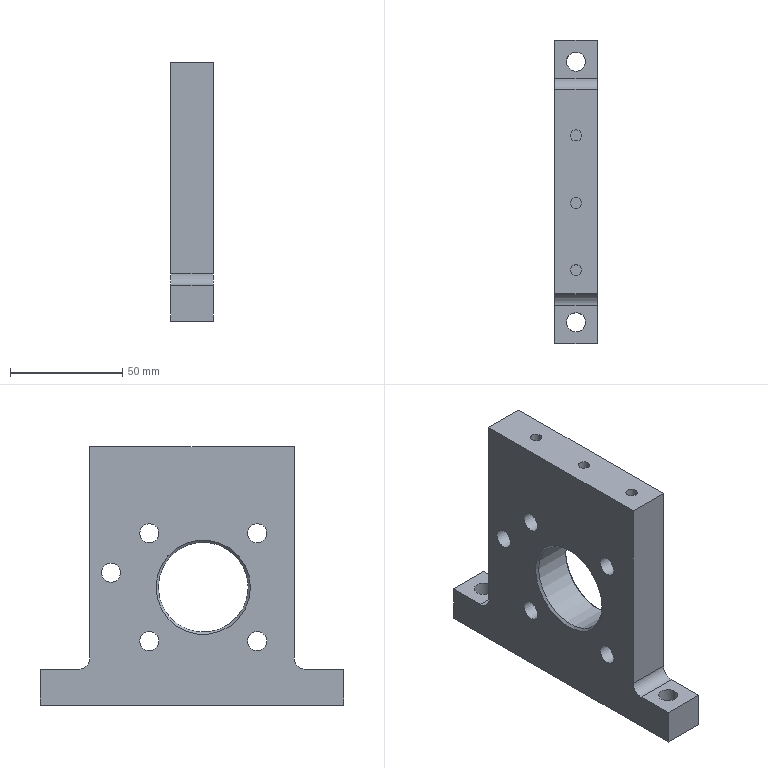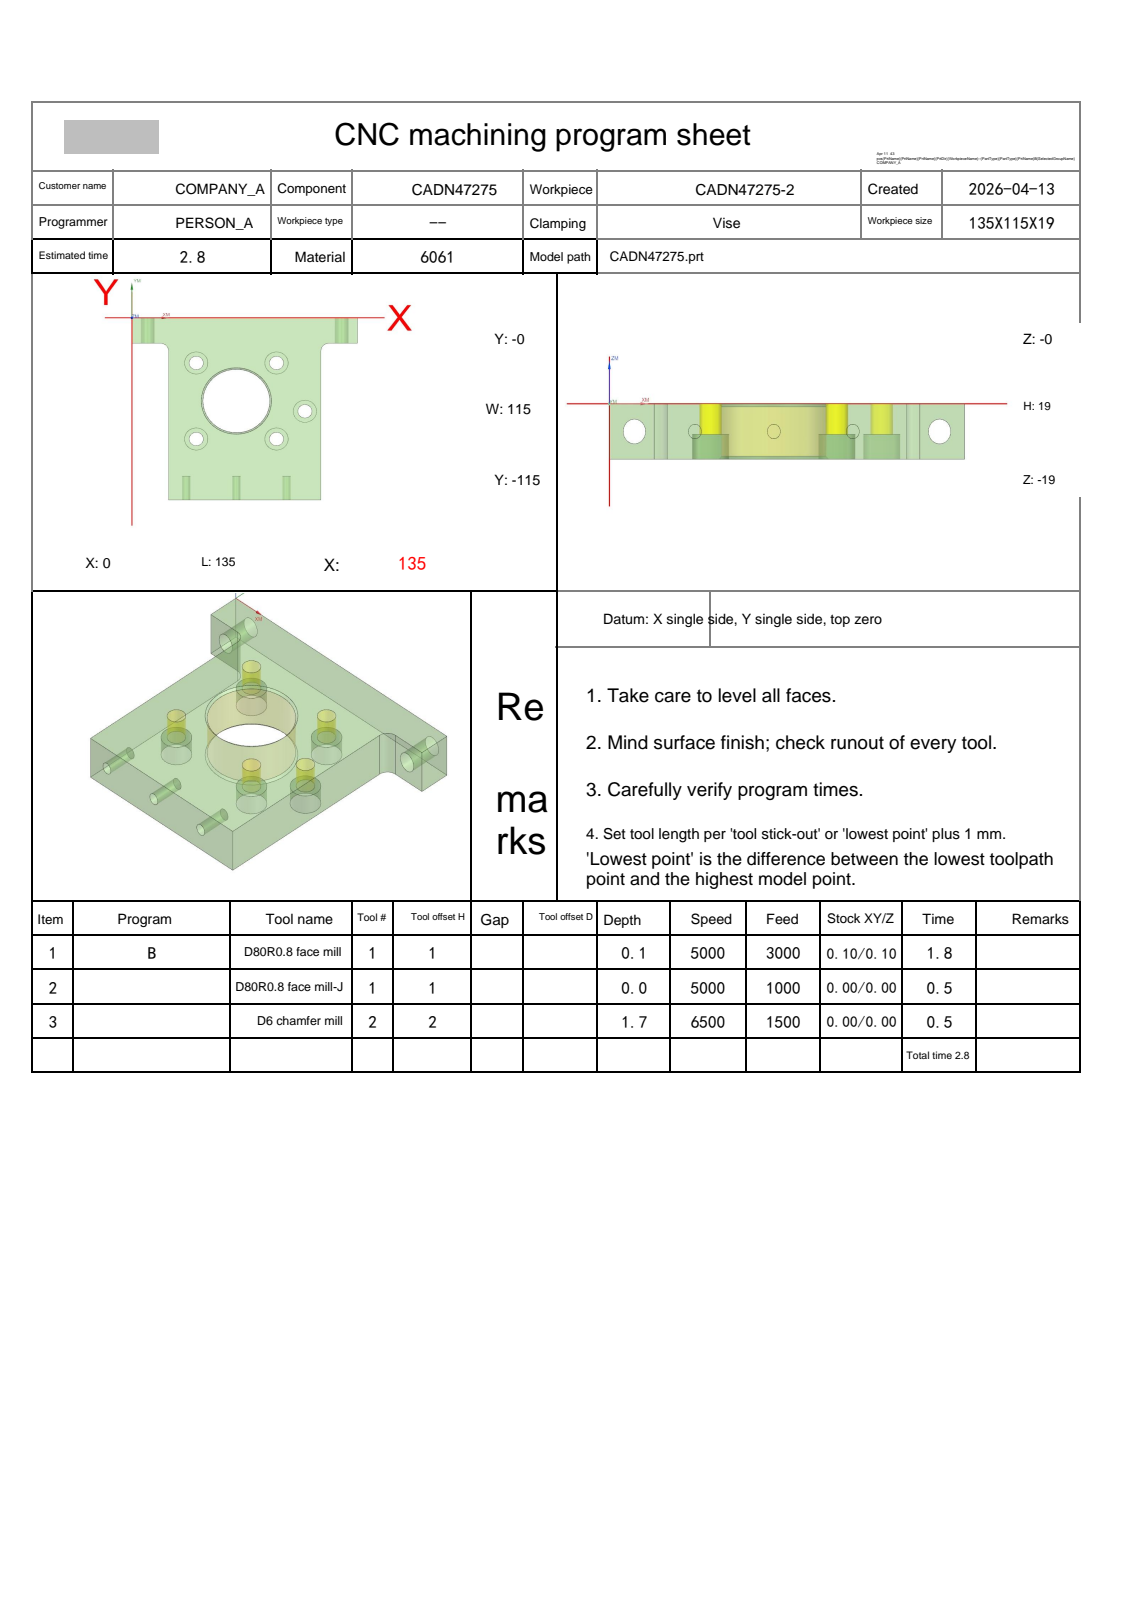NC program | NX | posted by the shop | part box 19 x 135 x 115 mm
Whole program:
%
O0001
(Machine time: 3.42 MIN)
(===Total Tool:2===)
(T1=D80R0.8 face mill D=80.  R=0.8  D-  H01 Z=-0.   )
(T2=D6 chamfer mill   D=6.   R=0.   D-  H02 Z=-1.7  )
G80 G90 G17 G49 G40
G91 G28 Z0
M01
N1 T01 M06
(D80R0.8 face mill  D=80. R=0.8 H=01 ce=0.10 di=0.10)
G00 G90 G54 X-52.097 Y-23.903 M03 S5000
G43 H01 Z20.
M08
Z7.009
G01 Z5.009 F3000.
X-40.097
X167.1
G02 X175.097 Y-31.9 I-.003 J-8.
G01 Y-53.303
G02 X173.357 Y-58.283 I-8. J.001
G01 X155.497 Y-80.721
G02 X149.243 Y-83.737 I-6.258 J4.984
G01 X-18.097
X-30.097
Z7.009
G00 X-52.097 Y-23.903
Z6.518
G01 Z4.518
X-40.097
X167.1
G02 X175.097 Y-31.9 I-.003 J-8.
G01 Y-53.303
G02 X173.357 Y-58.283 I-8. J.001
G01 X155.497 Y-80.721
G02 X149.243 Y-83.737 I-6.258 J4.984
G01 X-18.097
X-30.097
Z6.518
G00 X-52.097 Y-23.903
Z6.027
G01 Z4.027
X-40.097
X167.1
G02 X175.097 Y-31.9 I-.003 J-8.
G01 Y-53.303
G02 X173.357 Y-58.283 I-8. J.001
G01 X155.497 Y-80.721
G02 X149.243 Y-83.737 I-6.258 J4.984
G01 X-18.097
X-30.097
Z6.027
G00 X-52.097 Y-23.903
Z5.536
G01 Z3.536
X-40.097
X167.1
G02 X175.097 Y-31.9 I-.003 J-8.
G01 Y-53.303
G02 X173.357 Y-58.283 I-8. J.001
G01 X155.497 Y-80.721
G02 X149.243 Y-83.737 I-6.258 J4.984
G01 X-18.097
X-30.097
Z5.536
G00 X-52.097 Y-23.903
Z5.045
G01 Z3.045
X-40.097
X167.1
G02 X175.097 Y-31.9 I-.003 J-8.
G01 Y-53.303
G02 X173.357 Y-58.283 I-8. J.001
G01 X155.497 Y-80.721
G02 X149.243 Y-83.737 I-6.258 J4.984
G01 X-18.097
X-30.097
Z5.045
G00 X-52.097 Y-23.903
Z4.555
G01 Z2.555
X-40.097
X167.1
G02 X175.097 Y-31.9 I-.003 J-8.
G01 Y-53.303
G02 X173.357 Y-58.283 I-8. J.001
G01 X155.497 Y-80.721
G02 X149.243 Y-83.737 I-6.258 J4.984
G01 X-18.097
X-30.097
Z4.555
G00 X-52.097 Y-23.903
Z4.064
G01 Z2.064
X-40.097
X167.1
G02 X175.097 Y-31.9 I-.003 J-8.
G01 Y-53.303
G02 X173.357 Y-58.283 I-8. J.001
G01 X155.497 Y-80.721
G02 X149.243 Y-83.737 I-6.258 J4.984
G01 X-18.097
X-30.097
Z4.064
G00 X-52.097 Y-23.903
Z3.573
G01 Z1.573
X-40.097
X167.1
G02 X175.097 Y-31.9 I-.003 J-8.
G01 Y-53.303
G02 X173.357 Y-58.283 I-8. J.001
G01 X155.497 Y-80.721
G02 X149.243 Y-83.737 I-6.258 J4.984
G01 X-18.097
X-30.097
Z3.573
G00 X-52.097 Y-23.903
Z3.082
G01 Z1.082
X-40.097
X167.1
G02 X175.097 Y-31.9 I-.003 J-8.
G01 Y-53.303
G02 X173.357 Y-58.283 I-8. J.001
G01 X155.497 Y-80.721
G02 X149.243 Y-83.737 I-6.258 J4.984
G01 X-18.097
X-30.097
Z3.082
G00 X-52.097 Y-23.903
Z2.591
G01 Z.591
X-40.097
X167.1
G02 X175.097 Y-31.9 I-.003 J-8.
G01 Y-53.303
G02 X173.357 Y-58.283 I-8. J.001
G01 X155.497 Y-80.721
G02 X149.243 Y-83.737 I-6.258 J4.984
G01 X-18.097
X-30.097
Z2.591
G00 X-52.097 Y-23.903
Z2.1
G01 Z.1
X-40.097
X167.1
G02 X175.097 Y-31.9 I-.003 J-8.
G01 Y-53.303
G02 X173.357 Y-58.283 I-8. J.001
G01 X155.497 Y-80.721
G02 X149.243 Y-83.737 I-6.258 J4.984
G01 X-18.097
X-30.097
Z2.1
G00 Z20.
G91 G28 Z0.0
M05
M09
G91 G28 Z0.0
M01
N2 T01 M06
(D80R0.8 face mill-J  D=80. R=0.8 H=01 ce=0.00 di=0.00)
G00 G90 G54 X-51.999 Y-24.001 M03 S5000
G43 H01 Z20.
M08
Z2.
G01 Z0.0 F1000.
X-39.999
X167.002
G02 X174.999 Y-31.998 I-.003 J-8.
G01 Y-53.205
G02 X173.259 Y-58.185 I-8. J.001
G01 X155.399 Y-80.623
G02 X149.145 Y-83.639 I-6.258 J4.984
G01 X-17.999
X-29.999
Z2.
G00 Z20.
G91 G28 Z0.0
M05
M09
G91 G28 Z0.0
M01
N3 T02 M06
(D6 chamfer mill  D=6. R=0. H=02 ce=0.00 di=0.00)
G00 G90 G54 X67.114 Y1.227 M03 S6500
G43 H02 Z20.
M08
Z.172
G01 Z-1.199 F1500.
G03 X67.4 Y1.027 I1.286 J1.532
G01 X67.446 Y.997
X67.5 Y1.
X135.
G02 X136. Y0.0 I0.0 J-1.
G01 Y-16.
G02 X135. Y-17. I-1. J0.0
G01 X118.
G03 X114. Y-21. I0.0 J-4.
G01 Y-115.
G02 X113. Y-116. I-1. J0.0
G01 X22.
G02 X21. Y-115. I0.0 J1.
G01 Y-21.
G03 X17. Y-17. I-4. J0.0
G01 X0.0
G02 X-1. Y-16. I0.0 J1.
G01 Y0.0
G02 X0.0 Y1. I1. J0.0
G01 X67.5
X67.554 Y.997
X67.6 Y1.027
G03 X67.886 Y1.227 I-1. J1.732
G01 Z.172
G00 Z10.
X38.099 Y-31.553
Z.237
G01 Z-1.199
G03 X38.398 Y-31.731 I1.167 J1.624
G01 X38.446 Y-31.757
X38.5 Y-31.75
G03 X41.75 Y-28.5 I0.0 J3.25
X38.5 Y-25.25 I-3.25 J0.0
X35.25 Y-28.5 I0.0 J-3.25
X38.5 Y-31.75 I3.25 J0.0
G01 X38.554 Y-31.757
X38.602 Y-31.731
G03 X38.901 Y-31.553 I-.868 J1.802
G01 Z.237
G00 Z10.
X86.099
Z.237
G01 Z-1.199
G03 X86.398 Y-31.731 I1.167 J1.624
G01 X86.446 Y-31.757
X86.5 Y-31.75
G03 X89.75 Y-28.5 I0.0 J3.25
X86.5 Y-25.25 I-3.25 J0.0
X83.25 Y-28.5 I0.0 J-3.25
X86.5 Y-31.75 I3.25 J0.0
G01 X86.554 Y-31.757
X86.602 Y-31.731
G03 X86.901 Y-31.553 I-.868 J1.802
G01 Z.237
G00 Z10.
X103.099 Y-62.053
Z.237
G01 Z-1.199
G03 X103.398 Y-62.231 I1.167 J1.624
G01 X103.446 Y-62.257
X103.5 Y-62.25
G03 X106.75 Y-59. I0.0 J3.25
X103.5 Y-55.75 I-3.25 J0.0
X100.25 Y-59. I0.0 J-3.25
X103.5 Y-62.25 I3.25 J0.0
G01 X103.554 Y-62.257
X103.602 Y-62.231
G03 X103.901 Y-62.053 I-.868 J1.802
G01 Z.237
G00 Z10.
X86.099 Y-79.553
Z.237
G01 Z-1.199
G03 X86.398 Y-79.731 I1.167 J1.624
G01 X86.446 Y-79.757
X86.5 Y-79.75
G03 X89.75 Y-76.5 I0.0 J3.25
X86.5 Y-73.25 I-3.25 J0.0
X83.25 Y-76.5 I0.0 J-3.25
X86.5 Y-79.75 I3.25 J0.0
G01 X86.554 Y-79.757
X86.602 Y-79.731
G03 X86.901 Y-79.553 I-.868 J1.802
G01 Z.237
G00 Z10.
X38.901 Y-73.447
Z.237
G01 Z-1.199
G03 X38.602 Y-73.269 I-1.167 J-1.624
G01 X38.554 Y-73.243
X38.5 Y-73.25
G03 X35.25 Y-76.5 I0.0 J-3.25
X38.5 Y-79.75 I3.25 J0.0
X41.75 Y-76.5 I0.0 J3.25
X38.5 Y-73.25 I-3.25 J0.0
G01 X38.446 Y-73.243
X38.398 Y-73.269
G03 X38.099 Y-73.447 I.868 J-1.802
G01 Z.237
G00 Z20.
G00 G90 X63.7 Y-34.44 M03 S6500
Z20.
Z-.2
G01 Z-1.7 F1500.
Y-34.4
G03 X62.5 Y-33.2 I-1.2 J0.0
X43.2 Y-52.5 I0.0 J-19.3
X43.204 Y-52.888 I19.3 J0.0
X43.414 Y-55.365 I19.296 J.388
X43.474 Y-55.74 I19.086 J2.865
X44.717 Y-59.999 I19.026 J3.24
X45.893 Y-62.334 I17.783 J7.499
X46.059 Y-62.609 I16.607 J9.834
X62.5 Y-71.8 I16.441 J10.109
X81.8 Y-52.5 I0.0 J19.3
X62.5 Y-33.2 I-19.3 J0.0
X62.1 Y-33.204 I0.0 J-19.3
X60.925 Y-34.404 I.025 J-1.2
G01 Y-34.429
X60.926 Y-34.469
Z-.2
G00 Z20.
M05
M09
G91 G28 Z0.0
G91 G28 Y0.0
M30
%